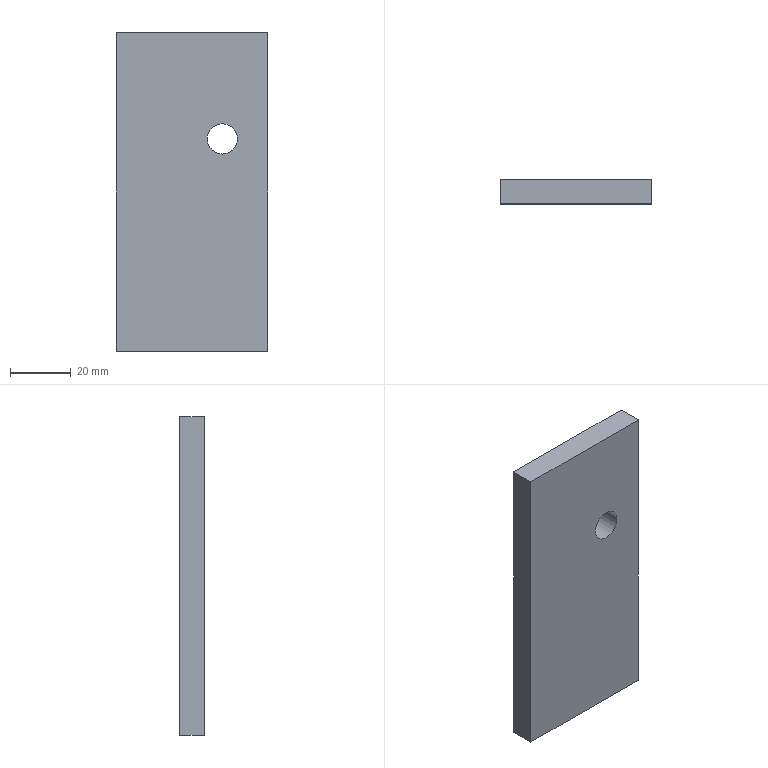Part | NX | features solid 2 | 1 solid | 7 faces | box 50 x 8 x 105 mm | volume 41372 mm3 | plane 6 | cylinder 1 | commonest cylinder face diameters 10 x1
STEP:
#1=CARTESIAN_POINT('',(475.,460.,-95.));
#2=VERTEX_POINT('',#1);
#3=CARTESIAN_POINT('',(475.,468.,-95.));
#4=VERTEX_POINT('',#3);
#5=CARTESIAN_POINT('',(475.,468.,-95.));
#6=DIRECTION('',(0.,-1.,0.));
#7=VECTOR('',#6,1000.);
#8=LINE('',#5,#7);
#9=EDGE_CURVE('',#2,#4,#8,.F.);
#10=ORIENTED_EDGE('',*,*,#9,.F.);
#11=CARTESIAN_POINT('',(425.,460.,-95.));
#12=VERTEX_POINT('',#11);
#13=CARTESIAN_POINT('',(475.,460.,-95.));
#14=DIRECTION('',(-1.,0.,0.));
#15=VECTOR('',#14,1000.);
#16=LINE('',#13,#15);
#17=EDGE_CURVE('',#2,#12,#16,.T.);
#18=ORIENTED_EDGE('',*,*,#17,.T.);
#19=CARTESIAN_POINT('',(425.,468.,-95.));
#20=VERTEX_POINT('',#19);
#21=CARTESIAN_POINT('',(425.,388.,-95.));
#22=DIRECTION('',(0.,-1.,0.));
#23=VECTOR('',#22,1000.);
#24=LINE('',#21,#23);
#25=EDGE_CURVE('',#12,#20,#24,.F.);
#26=ORIENTED_EDGE('',*,*,#25,.T.);
#27=CARTESIAN_POINT('',(475.,468.,-95.));
#28=DIRECTION('',(-1.,0.,0.));
#29=VECTOR('',#28,1000.);
#30=LINE('',#27,#29);
#31=EDGE_CURVE('',#4,#20,#30,.T.);
#32=ORIENTED_EDGE('',*,*,#31,.F.);
#33=EDGE_LOOP('',(#10,#18,#26,#32));
#34=FACE_BOUND('',#33,.T.);
#35=CARTESIAN_POINT('',(445.,388.,-95.));
#36=DIRECTION('',(0.,0.,-1.));
#37=DIRECTION('',(0.,1.,0.));
#38=AXIS2_PLACEMENT_3D('',#35,#36,#37);
#39=PLANE('',#38);
#40=ADVANCED_FACE('',(#34),#39,.T.);
#41=ORIENTED_EDGE('',*,*,#25,.F.);
#42=CARTESIAN_POINT('',(425.,460.,10.));
#43=VERTEX_POINT('',#42);
#44=CARTESIAN_POINT('',(425.,460.,-90.));
#45=DIRECTION('',(0.,0.,-1.));
#46=VECTOR('',#45,1000.);
#47=LINE('',#44,#46);
#48=EDGE_CURVE('',#12,#43,#47,.F.);
#49=ORIENTED_EDGE('',*,*,#48,.T.);
#50=CARTESIAN_POINT('',(425.,468.,10.));
#51=VERTEX_POINT('',#50);
#52=CARTESIAN_POINT('',(425.,460.,10.));
#53=DIRECTION('',(0.,1.,0.));
#54=VECTOR('',#53,1000.);
#55=LINE('',#52,#54);
#56=EDGE_CURVE('',#43,#51,#55,.T.);
#57=ORIENTED_EDGE('',*,*,#56,.T.);
#58=CARTESIAN_POINT('',(425.,468.,-90.));
#59=DIRECTION('',(0.,0.,-1.));
#60=VECTOR('',#59,1000.);
#61=LINE('',#58,#60);
#62=EDGE_CURVE('',#20,#51,#61,.F.);
#63=ORIENTED_EDGE('',*,*,#62,.F.);
#64=EDGE_LOOP('',(#41,#49,#57,#63));
#65=FACE_BOUND('',#64,.T.);
#66=CARTESIAN_POINT('',(425.,460.,-55.));
#67=DIRECTION('',(1.,0.,0.));
#68=DIRECTION('',(0.,0.,-1.));
#69=AXIS2_PLACEMENT_3D('',#66,#67,#68);
#70=PLANE('',#69);
#71=ADVANCED_FACE('',(#65),#70,.F.);
#72=ORIENTED_EDGE('',*,*,#56,.F.);
#73=CARTESIAN_POINT('',(475.,460.,10.));
#74=VERTEX_POINT('',#73);
#75=CARTESIAN_POINT('',(475.,460.,10.));
#76=DIRECTION('',(1.,0.,0.));
#77=VECTOR('',#76,1000.);
#78=LINE('',#75,#77);
#79=EDGE_CURVE('',#74,#43,#78,.F.);
#80=ORIENTED_EDGE('',*,*,#79,.F.);
#81=CARTESIAN_POINT('',(475.,468.,10.));
#82=VERTEX_POINT('',#81);
#83=CARTESIAN_POINT('',(475.,468.,10.));
#84=DIRECTION('',(0.,1.,0.));
#85=VECTOR('',#84,1000.);
#86=LINE('',#83,#85);
#87=EDGE_CURVE('',#74,#82,#86,.T.);
#88=ORIENTED_EDGE('',*,*,#87,.T.);
#89=CARTESIAN_POINT('',(475.,468.,10.));
#90=DIRECTION('',(1.,0.,0.));
#91=VECTOR('',#90,1000.);
#92=LINE('',#89,#91);
#93=EDGE_CURVE('',#82,#51,#92,.F.);
#94=ORIENTED_EDGE('',*,*,#93,.T.);
#95=EDGE_LOOP('',(#72,#80,#88,#94));
#96=FACE_BOUND('',#95,.T.);
#97=CARTESIAN_POINT('',(475.,468.,10.));
#98=DIRECTION('',(0.,0.,-1.));
#99=DIRECTION('',(-1.,0.,0.));
#100=AXIS2_PLACEMENT_3D('',#97,#98,#99);
#101=PLANE('',#100);
#102=ADVANCED_FACE('',(#96),#101,.F.);
#103=CARTESIAN_POINT('',(460.,468.,-30.));
#104=VERTEX_POINT('',#103);
#105=CARTESIAN_POINT('',(460.,468.,-25.));
#106=DIRECTION('',(0.,-1.,0.));
#107=DIRECTION('',(0.,0.,-1.));
#108=AXIS2_PLACEMENT_3D('',#105,#106,#107);
#109=CIRCLE('',#108,5.);
#110=EDGE_CURVE('',#104,#104,#109,.T.);
#111=ORIENTED_EDGE('',*,*,#110,.T.);
#112=EDGE_LOOP('',(#111));
#113=FACE_BOUND('',#112,.T.);
#114=ORIENTED_EDGE('',*,*,#93,.F.);
#115=CARTESIAN_POINT('',(475.,468.,-90.));
#116=DIRECTION('',(0.,0.,1.));
#117=VECTOR('',#116,1000.);
#118=LINE('',#115,#117);
#119=EDGE_CURVE('',#4,#82,#118,.T.);
#120=ORIENTED_EDGE('',*,*,#119,.F.);
#121=ORIENTED_EDGE('',*,*,#31,.T.);
#122=ORIENTED_EDGE('',*,*,#62,.T.);
#123=EDGE_LOOP('',(#114,#120,#121,#122));
#124=FACE_BOUND('',#123,.T.);
#125=CARTESIAN_POINT('',(475.,468.,-90.));
#126=DIRECTION('',(0.,1.,0.));
#127=DIRECTION('',(0.,0.,1.));
#128=AXIS2_PLACEMENT_3D('',#125,#126,#127);
#129=PLANE('',#128);
#130=ADVANCED_FACE('',(#113,#124),#129,.T.);
#131=CARTESIAN_POINT('',(475.,460.,-90.));
#132=DIRECTION('',(0.,0.,1.));
#133=VECTOR('',#132,1000.);
#134=LINE('',#131,#133);
#135=EDGE_CURVE('',#2,#74,#134,.T.);
#136=ORIENTED_EDGE('',*,*,#135,.F.);
#137=ORIENTED_EDGE('',*,*,#9,.T.);
#138=ORIENTED_EDGE('',*,*,#119,.T.);
#139=ORIENTED_EDGE('',*,*,#87,.F.);
#140=EDGE_LOOP('',(#136,#137,#138,#139));
#141=FACE_BOUND('',#140,.T.);
#142=CARTESIAN_POINT('',(475.,468.,-90.));
#143=DIRECTION('',(-1.,0.,0.));
#144=DIRECTION('',(0.,0.,1.));
#145=AXIS2_PLACEMENT_3D('',#142,#143,#144);
#146=PLANE('',#145);
#147=ADVANCED_FACE('',(#141),#146,.F.);
#148=CARTESIAN_POINT('',(460.,460.,-20.));
#149=VERTEX_POINT('',#148);
#150=CARTESIAN_POINT('',(460.,460.,-25.));
#151=DIRECTION('',(0.,1.,0.));
#152=DIRECTION('',(0.,0.,1.));
#153=AXIS2_PLACEMENT_3D('',#150,#151,#152);
#154=CIRCLE('',#153,5.);
#155=EDGE_CURVE('',#149,#149,#154,.T.);
#156=ORIENTED_EDGE('',*,*,#155,.T.);
#157=EDGE_LOOP('',(#156));
#158=FACE_BOUND('',#157,.T.);
#159=ORIENTED_EDGE('',*,*,#79,.T.);
#160=ORIENTED_EDGE('',*,*,#48,.F.);
#161=ORIENTED_EDGE('',*,*,#17,.F.);
#162=ORIENTED_EDGE('',*,*,#135,.T.);
#163=EDGE_LOOP('',(#159,#160,#161,#162));
#164=FACE_BOUND('',#163,.T.);
#165=CARTESIAN_POINT('',(475.,460.,-90.));
#166=DIRECTION('',(0.,1.,0.));
#167=DIRECTION('',(0.,0.,1.));
#168=AXIS2_PLACEMENT_3D('',#165,#166,#167);
#169=PLANE('',#168);
#170=ADVANCED_FACE('',(#158,#164),#169,.F.);
#171=ORIENTED_EDGE('',*,*,#110,.F.);
#172=EDGE_LOOP('',(#171));
#173=FACE_BOUND('',#172,.T.);
#174=ORIENTED_EDGE('',*,*,#155,.F.);
#175=EDGE_LOOP('',(#174));
#176=FACE_BOUND('',#175,.T.);
#177=CARTESIAN_POINT('',(460.,468.,-25.));
#178=DIRECTION('',(0.,-1.,0.));
#179=DIRECTION('',(0.,0.,-1.));
#180=AXIS2_PLACEMENT_3D('',#177,#178,#179);
#181=CYLINDRICAL_SURFACE('',#180,5.);
#182=ADVANCED_FACE('',(#173,#176),#181,.F.);
#183=CLOSED_SHELL('',(#40,#71,#102,#130,#147,#170,#182));
#184=MANIFOLD_SOLID_BREP('',#183);
#185=(LENGTH_UNIT()NAMED_UNIT(*)SI_UNIT(.MILLI.,.METRE.));
#186=UNCERTAINTY_MEASURE_WITH_UNIT(LENGTH_MEASURE(0.00001),#185,'','');
#187=(NAMED_UNIT(*)PLANE_ANGLE_UNIT()SI_UNIT($,.RADIAN.));
#188=(NAMED_UNIT(*)SI_UNIT($,.STERADIAN.)SOLID_ANGLE_UNIT());
#189=(GEOMETRIC_REPRESENTATION_CONTEXT(3)GLOBAL_UNCERTAINTY_ASSIGNED_CONTEXT((#186))GLOBAL_UNIT_ASSIGNED_CONTEXT((#185,#187,#188))REPRESENTATION_CONTEXT('',''));
#190=ADVANCED_BREP_SHAPE_REPRESENTATION('',(#184),#189);